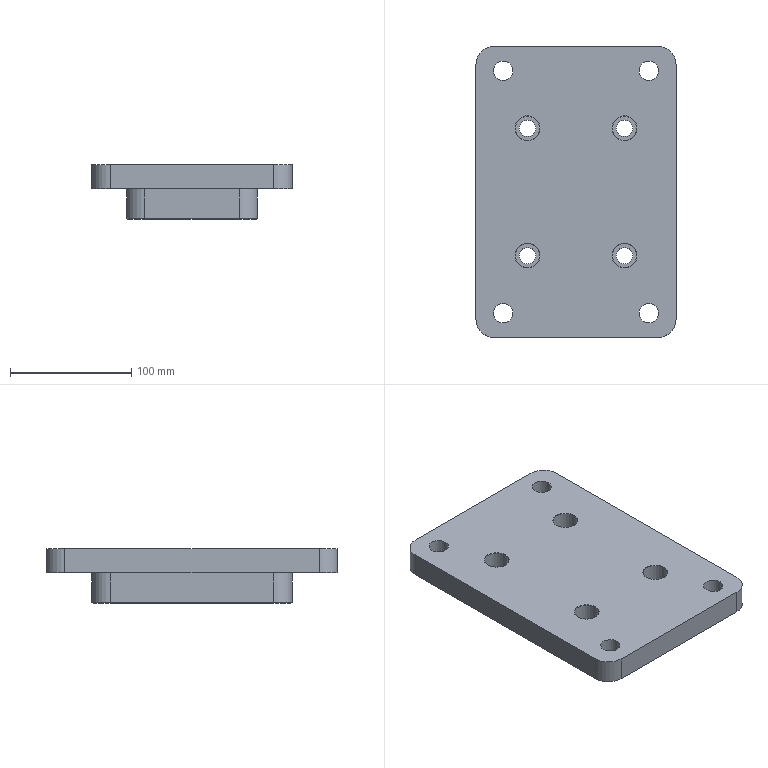NC program | NX | posted with a generic post | part box 165 x 240 x 45 mm
Lines 1 to 39 of 5916:
N10 G17 G21 G94 G90
(DRILLING , TOOL : ZXZ)
N12 T01 M6
N14 G54
N16 G17 G0 G90 X100. Y60. S5000 M3
N18 G43 Z30. H1
N20 G94 G81 G98 Z-1. F250. R3.
N22 X52.5 Y40.
N24 X100. Y-60.
N26 X52.5 Y-40.
N28 X-52.5
N30 X-100. Y-60.
N32 X-52.5 Y40.
N34 X-100. Y60.
N36 G80
N38 G0 X-100. Y60. Z30.
N40 M5
(DRILLING_COPY , TOOL : 13.5ZT)
N42 T13 M6
N44 G54
N46 G17 G0 G90 X100. Y60. S2000 M3
N48 G43 Z30. H13
N50 G94 G83 G98 Z-25.556 F200. Q2. R3.
N52 X52.5 Y40. Z-50.556
N54 X100. Y-60. Z-25.556
N56 X52.5 Y-40. Z-50.556
N58 X-52.5
N60 X-100. Y-60. Z-25.556
N62 X-52.5 Y40. Z-50.556
N64 X-100. Y60. Z-25.556
N66 G80
N68 G0 X-100. Y60. Z30.
N70 M5